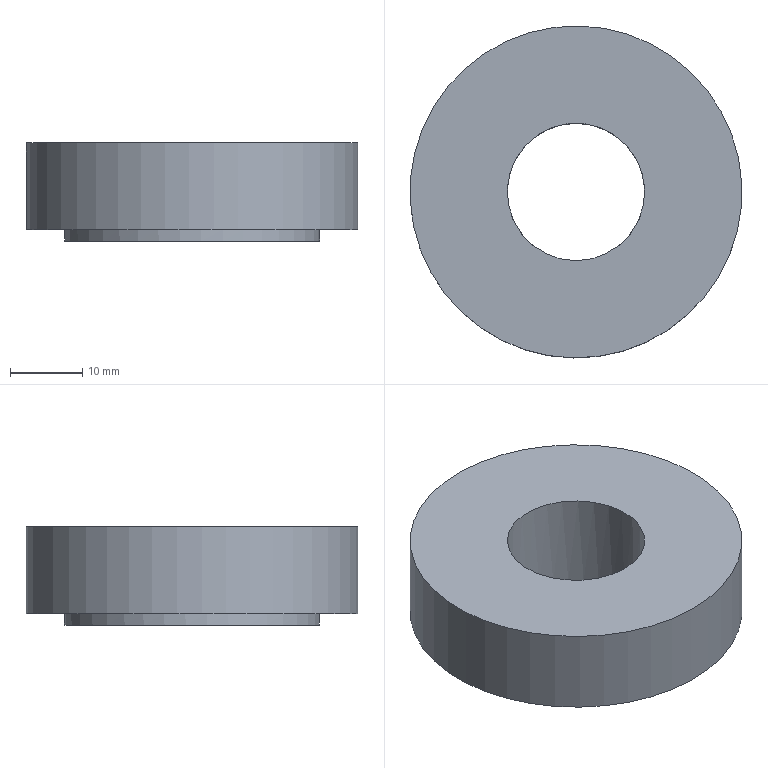Part | NX | features solid 2 | 1 solid | 6 faces | box 46 x 46 x 13.602 mm | volume 17638 mm3 | cylinder 3 | plane 3 | commonest cylinder face diameters 19.05 x1 35.368 x1 46 x1
STEP:
#1=CARTESIAN_POINT('',(-471.467,-977.315,-33.985));
#2=VERTEX_POINT('',#1);
#3=CARTESIAN_POINT('',(-484.114,-958.104,-33.986));
#4=DIRECTION('',(-0.0000242,0.00003327,1.));
#5=DIRECTION('',(0.5498,-0.8353,0.00004109));
#6=AXIS2_PLACEMENT_3D('',#3,#4,#5);
#7=CIRCLE('',#6,23.);
#8=EDGE_CURVE('',#2,#2,#7,.T.);
#9=ORIENTED_EDGE('',*,*,#8,.T.);
#10=EDGE_LOOP('',(#9));
#11=FACE_BOUND('',#10,.T.);
#12=CARTESIAN_POINT('',(-471.468,-977.315,-21.985));
#13=VERTEX_POINT('',#12);
#14=CARTESIAN_POINT('',(-484.114,-958.104,-21.986));
#15=DIRECTION('',(-0.0000242,0.00003327,1.));
#16=DIRECTION('',(0.5498,-0.8353,0.00004109));
#17=AXIS2_PLACEMENT_3D('',#14,#15,#16);
#18=CIRCLE('',#17,23.);
#19=EDGE_CURVE('',#13,#13,#18,.T.);
#20=ORIENTED_EDGE('',*,*,#19,.F.);
#21=EDGE_LOOP('',(#20));
#22=FACE_BOUND('',#21,.T.);
#23=CARTESIAN_POINT('',(-484.113,-958.105,-73.319));
#24=DIRECTION('',(-0.0000242,0.00003327,1.));
#25=DIRECTION('',(0.5498,-0.8353,0.00004109));
#26=AXIS2_PLACEMENT_3D('',#23,#24,#25);
#27=CYLINDRICAL_SURFACE('',#26,23.);
#28=ADVANCED_FACE('',(#11,#22),#27,.T.);
#29=CARTESIAN_POINT('',(-474.39,-972.875,-33.985));
#30=VERTEX_POINT('',#29);
#31=CARTESIAN_POINT('',(-484.114,-958.104,-33.986));
#32=DIRECTION('',(-0.0000242,0.00003327,1.));
#33=DIRECTION('',(0.5498,-0.8353,0.00004109));
#34=AXIS2_PLACEMENT_3D('',#31,#32,#33);
#35=CIRCLE('',#34,17.684);
#36=EDGE_CURVE('',#30,#30,#35,.T.);
#37=ORIENTED_EDGE('',*,*,#36,.T.);
#38=EDGE_LOOP('',(#37));
#39=FACE_BOUND('',#38,.T.);
#40=ORIENTED_EDGE('',*,*,#8,.F.);
#41=EDGE_LOOP('',(#40));
#42=FACE_BOUND('',#41,.T.);
#43=CARTESIAN_POINT('',(-501.654,-969.651,-33.986));
#44=DIRECTION('',(0.0000242,-0.00003327,-1.));
#45=DIRECTION('',(-0.5498,0.8353,-0.00004109));
#46=AXIS2_PLACEMENT_3D('',#43,#44,#45);
#47=PLANE('',#46);
#48=ADVANCED_FACE('',(#39,#42),#47,.T.);
#49=CARTESIAN_POINT('',(-484.114,-940.42,-35.586));
#50=VERTEX_POINT('',#49);
#51=CARTESIAN_POINT('',(-484.114,-958.104,-35.586));
#52=DIRECTION('',(0.0000242,-0.00003327,-1.));
#53=DIRECTION('',(0.,1.,-0.00003327));
#54=AXIS2_PLACEMENT_3D('',#51,#52,#53);
#55=CIRCLE('',#54,17.684);
#56=EDGE_CURVE('',#50,#50,#55,.F.);
#57=ORIENTED_EDGE('',*,*,#56,.T.);
#58=EDGE_LOOP('',(#57));
#59=FACE_BOUND('',#58,.T.);
#60=ORIENTED_EDGE('',*,*,#36,.F.);
#61=EDGE_LOOP('',(#60));
#62=FACE_BOUND('',#61,.T.);
#63=CARTESIAN_POINT('',(-484.113,-958.105,-73.319));
#64=DIRECTION('',(-0.0000242,0.00003327,1.));
#65=DIRECTION('',(0.5498,-0.8353,0.00004109));
#66=AXIS2_PLACEMENT_3D('',#63,#64,#65);
#67=CYLINDRICAL_SURFACE('',#66,17.684);
#68=ADVANCED_FACE('',(#59,#62),#67,.T.);
#69=CARTESIAN_POINT('',(-484.114,-948.579,-35.586));
#70=VERTEX_POINT('',#69);
#71=CARTESIAN_POINT('',(-484.114,-958.104,-35.586));
#72=DIRECTION('',(0.0000242,-0.00003327,-1.));
#73=DIRECTION('',(0.,1.,-0.00003327));
#74=AXIS2_PLACEMENT_3D('',#71,#72,#73);
#75=CIRCLE('',#74,9.525);
#76=EDGE_CURVE('',#70,#70,#75,.F.);
#77=ORIENTED_EDGE('',*,*,#76,.T.);
#78=EDGE_LOOP('',(#77));
#79=FACE_BOUND('',#78,.T.);
#80=ORIENTED_EDGE('',*,*,#56,.F.);
#81=EDGE_LOOP('',(#80));
#82=FACE_BOUND('',#81,.T.);
#83=CARTESIAN_POINT('',(-498.884,-967.827,-35.586));
#84=DIRECTION('',(0.0000242,-0.00003327,-1.));
#85=DIRECTION('',(-0.5498,0.8353,-0.00004109));
#86=AXIS2_PLACEMENT_3D('',#83,#84,#85);
#87=PLANE('',#86);
#88=ADVANCED_FACE('',(#79,#82),#87,.T.);
#89=CARTESIAN_POINT('',(-484.114,-967.629,-21.986));
#90=VERTEX_POINT('',#89);
#91=CARTESIAN_POINT('',(-484.114,-958.104,-21.986));
#92=DIRECTION('',(-0.0000242,0.00003327,1.));
#93=DIRECTION('',(0.,-1.,0.00003327));
#94=AXIS2_PLACEMENT_3D('',#91,#92,#93);
#95=CIRCLE('',#94,9.525);
#96=EDGE_CURVE('',#90,#90,#95,.T.);
#97=ORIENTED_EDGE('',*,*,#96,.T.);
#98=EDGE_LOOP('',(#97));
#99=FACE_BOUND('',#98,.T.);
#100=ORIENTED_EDGE('',*,*,#76,.F.);
#101=EDGE_LOOP('',(#100));
#102=FACE_BOUND('',#101,.T.);
#103=CARTESIAN_POINT('',(-484.113,-958.105,-73.319));
#104=DIRECTION('',(-0.0000242,0.00003327,1.));
#105=DIRECTION('',(0.5498,-0.8353,0.00004109));
#106=AXIS2_PLACEMENT_3D('',#103,#104,#105);
#107=CYLINDRICAL_SURFACE('',#106,9.525);
#108=ADVANCED_FACE('',(#99,#102),#107,.F.);
#109=ORIENTED_EDGE('',*,*,#19,.T.);
#110=EDGE_LOOP('',(#109));
#111=FACE_BOUND('',#110,.T.);
#112=ORIENTED_EDGE('',*,*,#96,.F.);
#113=EDGE_LOOP('',(#112));
#114=FACE_BOUND('',#113,.T.);
#115=CARTESIAN_POINT('',(-499.984,-968.551,-21.986));
#116=DIRECTION('',(-0.0000242,0.00003327,1.));
#117=DIRECTION('',(0.5498,-0.8353,0.00004109));
#118=AXIS2_PLACEMENT_3D('',#115,#116,#117);
#119=PLANE('',#118);
#120=ADVANCED_FACE('',(#111,#114),#119,.T.);
#121=CLOSED_SHELL('',(#28,#48,#68,#88,#108,#120));
#122=MANIFOLD_SOLID_BREP('',#121);
#123=(LENGTH_UNIT()NAMED_UNIT(*)SI_UNIT(.MILLI.,.METRE.));
#124=UNCERTAINTY_MEASURE_WITH_UNIT(LENGTH_MEASURE(0.00001),#123,'','');
#125=(NAMED_UNIT(*)PLANE_ANGLE_UNIT()SI_UNIT($,.RADIAN.));
#126=(NAMED_UNIT(*)SI_UNIT($,.STERADIAN.)SOLID_ANGLE_UNIT());
#127=(GEOMETRIC_REPRESENTATION_CONTEXT(3)GLOBAL_UNCERTAINTY_ASSIGNED_CONTEXT((#124))GLOBAL_UNIT_ASSIGNED_CONTEXT((#123,#125,#126))REPRESENTATION_CONTEXT('',''));
#128=ADVANCED_BREP_SHAPE_REPRESENTATION('',(#122),#127);